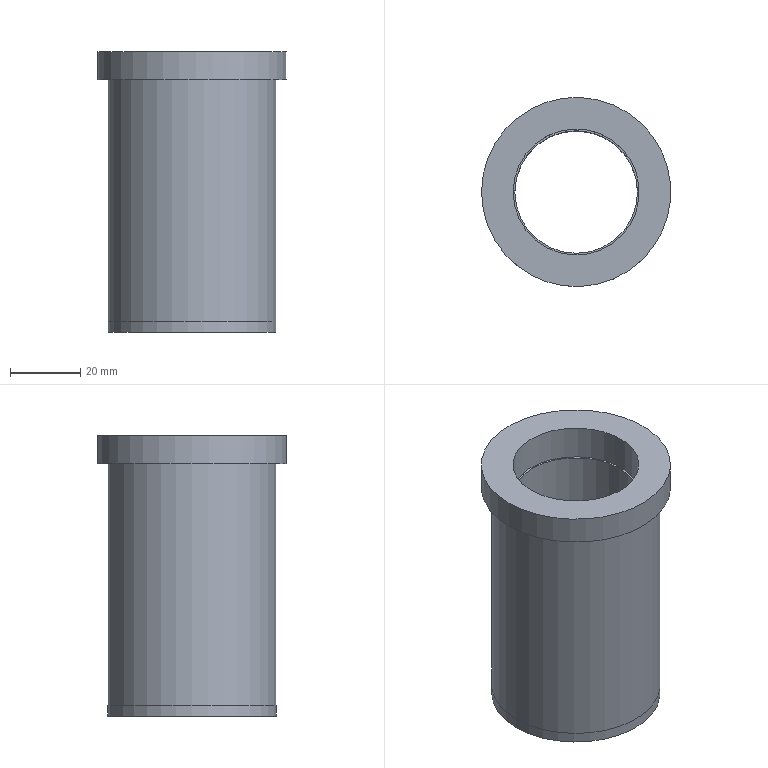Part | STEP file | 1_id474_xmt_txt | 1 solid | 10 faces | box 54 x 54 x 80 mm | volume 71084 mm3 | cylinder 5 | plane 5 | commonest cylinder face diameters 35 x1 36 x1 48 x1 48.005 x1 54 x1
STEP:
#1=CARTESIAN_POINT('',(-189.,302.,101.));
#2=VERTEX_POINT('',#1);
#3=CARTESIAN_POINT('',(-162.,302.,101.));
#4=DIRECTION('',(0.,0.,1.));
#5=DIRECTION('',(-1.,0.,0.));
#6=AXIS2_PLACEMENT_3D('',#3,#4,#5);
#7=CIRCLE('',#6,27.);
#8=EDGE_CURVE('',#2,#2,#7,.T.);
#9=ORIENTED_EDGE('',*,*,#8,.F.);
#10=EDGE_LOOP('',(#9));
#11=FACE_BOUND('',#10,.T.);
#12=CARTESIAN_POINT('',(-189.,302.,93.));
#13=VERTEX_POINT('',#12);
#14=CARTESIAN_POINT('',(-162.,302.,93.));
#15=DIRECTION('',(0.,0.,-1.));
#16=DIRECTION('',(-1.,0.,0.));
#17=AXIS2_PLACEMENT_3D('',#14,#15,#16);
#18=CIRCLE('',#17,27.);
#19=EDGE_CURVE('',#13,#13,#18,.T.);
#20=ORIENTED_EDGE('',*,*,#19,.F.);
#21=EDGE_LOOP('',(#20));
#22=FACE_BOUND('',#21,.T.);
#23=CARTESIAN_POINT('',(-162.,302.,97.));
#24=DIRECTION('',(0.,0.,-1.));
#25=DIRECTION('',(1.,0.,0.));
#26=AXIS2_PLACEMENT_3D('',#23,#24,#25);
#27=CYLINDRICAL_SURFACE('',#26,27.);
#28=ADVANCED_FACE('',(#11,#22),#27,.T.);
#29=CARTESIAN_POINT('',(-186.,302.,93.));
#30=VERTEX_POINT('',#29);
#31=CARTESIAN_POINT('',(-162.,302.,93.));
#32=DIRECTION('',(0.,0.,1.));
#33=DIRECTION('',(-1.,0.,0.));
#34=AXIS2_PLACEMENT_3D('',#31,#32,#33);
#35=CIRCLE('',#34,24.);
#36=EDGE_CURVE('',#30,#30,#35,.T.);
#37=ORIENTED_EDGE('',*,*,#36,.F.);
#38=EDGE_LOOP('',(#37));
#39=FACE_BOUND('',#38,.T.);
#40=CARTESIAN_POINT('',(-186.,302.,24.));
#41=VERTEX_POINT('',#40);
#42=CARTESIAN_POINT('',(-162.,302.,24.));
#43=DIRECTION('',(0.,0.,1.));
#44=DIRECTION('',(-1.,0.,0.));
#45=AXIS2_PLACEMENT_3D('',#42,#43,#44);
#46=CIRCLE('',#45,24.);
#47=EDGE_CURVE('',#41,#41,#46,.T.);
#48=ORIENTED_EDGE('',*,*,#47,.T.);
#49=EDGE_LOOP('',(#48));
#50=FACE_BOUND('',#49,.T.);
#51=CARTESIAN_POINT('',(-162.,302.,57.));
#52=DIRECTION('',(0.,0.,-1.));
#53=DIRECTION('',(1.,0.,0.));
#54=AXIS2_PLACEMENT_3D('',#51,#52,#53);
#55=CYLINDRICAL_SURFACE('',#54,24.);
#56=ADVANCED_FACE('',(#39,#50),#55,.T.);
#57=CARTESIAN_POINT('',(-180.,302.,91.));
#58=VERTEX_POINT('',#57);
#59=CARTESIAN_POINT('',(-162.,302.,91.));
#60=DIRECTION('',(0.,0.,-1.));
#61=DIRECTION('',(-1.,0.,0.));
#62=AXIS2_PLACEMENT_3D('',#59,#60,#61);
#63=CIRCLE('',#62,18.);
#64=EDGE_CURVE('',#58,#58,#63,.T.);
#65=ORIENTED_EDGE('',*,*,#64,.T.);
#66=EDGE_LOOP('',(#65));
#67=FACE_BOUND('',#66,.T.);
#68=CARTESIAN_POINT('',(-180.,302.,101.));
#69=VERTEX_POINT('',#68);
#70=CARTESIAN_POINT('',(-162.,302.,101.));
#71=DIRECTION('',(0.,0.,-1.));
#72=DIRECTION('',(-1.,0.,0.));
#73=AXIS2_PLACEMENT_3D('',#70,#71,#72);
#74=CIRCLE('',#73,18.);
#75=EDGE_CURVE('',#69,#69,#74,.T.);
#76=ORIENTED_EDGE('',*,*,#75,.F.);
#77=EDGE_LOOP('',(#76));
#78=FACE_BOUND('',#77,.T.);
#79=CARTESIAN_POINT('',(-162.,302.,96.));
#80=DIRECTION('',(0.,0.,-1.));
#81=DIRECTION('',(1.,0.,0.));
#82=AXIS2_PLACEMENT_3D('',#79,#80,#81);
#83=CYLINDRICAL_SURFACE('',#82,18.);
#84=ADVANCED_FACE('',(#67,#78),#83,.F.);
#85=CARTESIAN_POINT('',(-186.002,302.,24.));
#86=VERTEX_POINT('',#85);
#87=CARTESIAN_POINT('',(-162.,302.,24.));
#88=DIRECTION('',(0.,0.,1.));
#89=DIRECTION('',(-1.,0.,0.));
#90=AXIS2_PLACEMENT_3D('',#87,#88,#89);
#91=CIRCLE('',#90,24.003);
#92=EDGE_CURVE('',#86,#86,#91,.T.);
#93=ORIENTED_EDGE('',*,*,#92,.F.);
#94=EDGE_LOOP('',(#93));
#95=FACE_BOUND('',#94,.T.);
#96=CARTESIAN_POINT('',(-186.002,302.,21.));
#97=VERTEX_POINT('',#96);
#98=CARTESIAN_POINT('',(-162.,302.,21.));
#99=DIRECTION('',(0.,0.,-1.));
#100=DIRECTION('',(-1.,0.,0.));
#101=AXIS2_PLACEMENT_3D('',#98,#99,#100);
#102=CIRCLE('',#101,24.003);
#103=EDGE_CURVE('',#97,#97,#102,.T.);
#104=ORIENTED_EDGE('',*,*,#103,.F.);
#105=EDGE_LOOP('',(#104));
#106=FACE_BOUND('',#105,.T.);
#107=CARTESIAN_POINT('',(-162.,302.,22.5));
#108=DIRECTION('',(0.,0.,-1.));
#109=DIRECTION('',(1.,0.,0.));
#110=AXIS2_PLACEMENT_3D('',#107,#108,#109);
#111=CYLINDRICAL_SURFACE('',#110,24.003);
#112=ADVANCED_FACE('',(#95,#106),#111,.T.);
#113=CARTESIAN_POINT('',(-179.5,302.,21.));
#114=VERTEX_POINT('',#113);
#115=CARTESIAN_POINT('',(-162.,302.,21.));
#116=DIRECTION('',(0.,0.,1.));
#117=DIRECTION('',(-1.,0.,0.));
#118=AXIS2_PLACEMENT_3D('',#115,#116,#117);
#119=CIRCLE('',#118,17.5);
#120=EDGE_CURVE('',#114,#114,#119,.T.);
#121=ORIENTED_EDGE('',*,*,#120,.F.);
#122=EDGE_LOOP('',(#121));
#123=FACE_BOUND('',#122,.T.);
#124=CARTESIAN_POINT('',(-179.5,302.,91.));
#125=VERTEX_POINT('',#124);
#126=CARTESIAN_POINT('',(-162.,302.,91.));
#127=DIRECTION('',(0.,0.,-1.));
#128=DIRECTION('',(-1.,0.,0.));
#129=AXIS2_PLACEMENT_3D('',#126,#127,#128);
#130=CIRCLE('',#129,17.5);
#131=EDGE_CURVE('',#125,#125,#130,.T.);
#132=ORIENTED_EDGE('',*,*,#131,.F.);
#133=EDGE_LOOP('',(#132));
#134=FACE_BOUND('',#133,.T.);
#135=CARTESIAN_POINT('',(-162.,302.,56.));
#136=DIRECTION('',(0.,0.,-1.));
#137=DIRECTION('',(1.,0.,0.));
#138=AXIS2_PLACEMENT_3D('',#135,#136,#137);
#139=CYLINDRICAL_SURFACE('',#138,17.5);
#140=ADVANCED_FACE('',(#123,#134),#139,.F.);
#141=ORIENTED_EDGE('',*,*,#92,.T.);
#142=EDGE_LOOP('',(#141));
#143=FACE_BOUND('',#142,.T.);
#144=ORIENTED_EDGE('',*,*,#47,.F.);
#145=EDGE_LOOP('',(#144));
#146=FACE_BOUND('',#145,.T.);
#147=CARTESIAN_POINT('',(-162.,302.,24.));
#148=DIRECTION('',(0.,0.,1.));
#149=DIRECTION('',(-1.,0.,0.));
#150=AXIS2_PLACEMENT_3D('',#147,#148,#149);
#151=PLANE('',#150);
#152=ADVANCED_FACE('',(#143,#146),#151,.T.);
#153=ORIENTED_EDGE('',*,*,#131,.T.);
#154=EDGE_LOOP('',(#153));
#155=FACE_BOUND('',#154,.T.);
#156=ORIENTED_EDGE('',*,*,#64,.F.);
#157=EDGE_LOOP('',(#156));
#158=FACE_BOUND('',#157,.T.);
#159=CARTESIAN_POINT('',(-162.,302.,91.));
#160=DIRECTION('',(0.,0.,-1.));
#161=DIRECTION('',(1.,0.,0.));
#162=AXIS2_PLACEMENT_3D('',#159,#160,#161);
#163=PLANE('',#162);
#164=ADVANCED_FACE('',(#155,#158),#163,.F.);
#165=ORIENTED_EDGE('',*,*,#120,.T.);
#166=EDGE_LOOP('',(#165));
#167=FACE_BOUND('',#166,.T.);
#168=ORIENTED_EDGE('',*,*,#103,.T.);
#169=EDGE_LOOP('',(#168));
#170=FACE_BOUND('',#169,.T.);
#171=CARTESIAN_POINT('',(-162.,302.,21.));
#172=DIRECTION('',(0.,0.,-1.));
#173=DIRECTION('',(1.,0.,0.));
#174=AXIS2_PLACEMENT_3D('',#171,#172,#173);
#175=PLANE('',#174);
#176=ADVANCED_FACE('',(#167,#170),#175,.T.);
#177=ORIENTED_EDGE('',*,*,#75,.T.);
#178=EDGE_LOOP('',(#177));
#179=FACE_BOUND('',#178,.T.);
#180=ORIENTED_EDGE('',*,*,#8,.T.);
#181=EDGE_LOOP('',(#180));
#182=FACE_BOUND('',#181,.T.);
#183=CARTESIAN_POINT('',(-162.,302.,101.));
#184=DIRECTION('',(0.,0.,1.));
#185=DIRECTION('',(-1.,0.,0.));
#186=AXIS2_PLACEMENT_3D('',#183,#184,#185);
#187=PLANE('',#186);
#188=ADVANCED_FACE('',(#179,#182),#187,.T.);
#189=ORIENTED_EDGE('',*,*,#36,.T.);
#190=EDGE_LOOP('',(#189));
#191=FACE_BOUND('',#190,.T.);
#192=ORIENTED_EDGE('',*,*,#19,.T.);
#193=EDGE_LOOP('',(#192));
#194=FACE_BOUND('',#193,.T.);
#195=CARTESIAN_POINT('',(-162.,302.,93.));
#196=DIRECTION('',(0.,0.,-1.));
#197=DIRECTION('',(1.,0.,0.));
#198=AXIS2_PLACEMENT_3D('',#195,#196,#197);
#199=PLANE('',#198);
#200=ADVANCED_FACE('',(#191,#194),#199,.T.);
#201=CLOSED_SHELL('',(#28,#56,#84,#112,#140,#152,#164,#176,#188,#200));
#202=MANIFOLD_SOLID_BREP('',#201);
#203=(LENGTH_UNIT()NAMED_UNIT(*)SI_UNIT(.MILLI.,.METRE.));
#204=UNCERTAINTY_MEASURE_WITH_UNIT(LENGTH_MEASURE(0.00002),#203,'','');
#205=(NAMED_UNIT(*)PLANE_ANGLE_UNIT()SI_UNIT($,.RADIAN.));
#206=PLANE_ANGLE_MEASURE_WITH_UNIT(PLANE_ANGLE_MEASURE(0.01745),#205);
#207=DIMENSIONAL_EXPONENTS(0.,0.,0.,0.,0.,0.,0.);
#208=(CONVERSION_BASED_UNIT('DEGREE',#206)NAMED_UNIT(#207)PLANE_ANGLE_UNIT());
#209=(NAMED_UNIT(*)SI_UNIT($,.STERADIAN.)SOLID_ANGLE_UNIT());
#210=(GEOMETRIC_REPRESENTATION_CONTEXT(3)GLOBAL_UNCERTAINTY_ASSIGNED_CONTEXT((#204))GLOBAL_UNIT_ASSIGNED_CONTEXT((#203,#208,#209))REPRESENTATION_CONTEXT('',''));
#211=ADVANCED_BREP_SHAPE_REPRESENTATION('',(#202),#210);